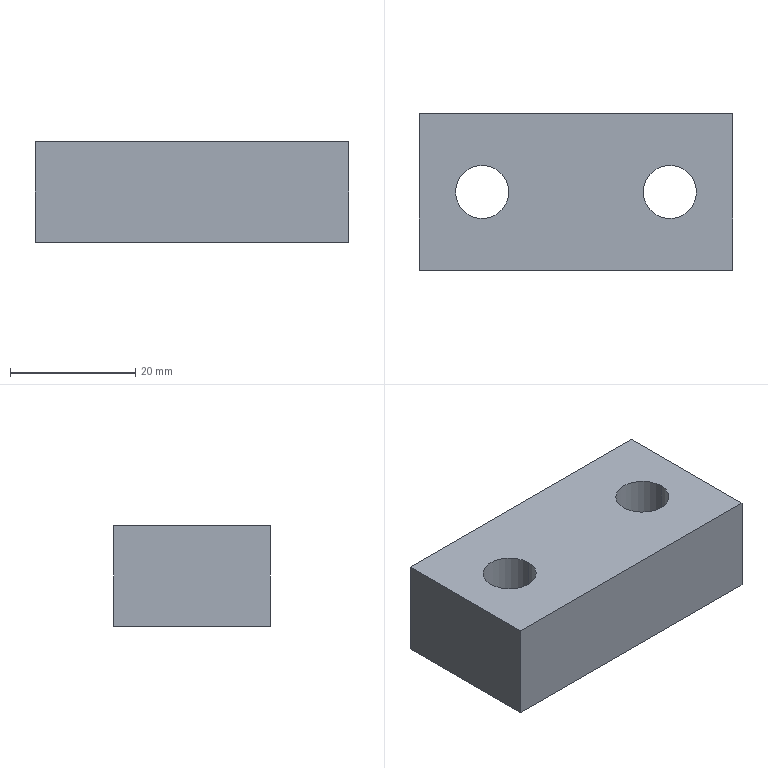Part | SolidWorks | features FlatPattern 1, HoleWzd 1, SMBaseFlange 1, SheetMetal 1 | 1 solid | 10 faces | box 50 x 25 x 16 mm | volume 18184 mm3 | plane 6 | cylinder 4 | commonest cylinder face diameters 8.5 x4
STEP:
#1=CARTESIAN_POINT('',(35.75,-12.5,-16.));
#2=VERTEX_POINT('',#1);
#3=CARTESIAN_POINT('',(44.25,-12.5,-16.));
#4=VERTEX_POINT('',#3);
#5=CARTESIAN_POINT('',(40.,-12.5,-16.));
#6=DIRECTION('',(0.,0.,1.));
#7=DIRECTION('',(1.,0.,0.));
#8=AXIS2_PLACEMENT_3D('',#5,#6,#7);
#9=CIRCLE('',#8,4.25);
#10=EDGE_CURVE('',#2,#4,#9,.T.);
#11=ORIENTED_EDGE('',*,*,#10,.F.);
#12=CARTESIAN_POINT('',(35.75,-12.5,0.));
#13=VERTEX_POINT('',#12);
#14=CARTESIAN_POINT('',(35.75,-12.5,0.));
#15=DIRECTION('',(0.,0.,1.));
#16=VECTOR('',#15,1000.);
#17=LINE('',#14,#16);
#18=EDGE_CURVE('',#2,#13,#17,.T.);
#19=ORIENTED_EDGE('',*,*,#18,.T.);
#20=CARTESIAN_POINT('',(44.25,-12.5,0.));
#21=VERTEX_POINT('',#20);
#22=CARTESIAN_POINT('',(40.,-12.5,0.));
#23=DIRECTION('',(0.,0.,1.));
#24=DIRECTION('',(1.,0.,0.));
#25=AXIS2_PLACEMENT_3D('',#22,#23,#24);
#26=CIRCLE('',#25,4.25);
#27=EDGE_CURVE('',#13,#21,#26,.T.);
#28=ORIENTED_EDGE('',*,*,#27,.T.);
#29=CARTESIAN_POINT('',(44.25,-12.5,0.));
#30=DIRECTION('',(0.,0.,1.));
#31=VECTOR('',#30,1000.);
#32=LINE('',#29,#31);
#33=EDGE_CURVE('',#4,#21,#32,.T.);
#34=ORIENTED_EDGE('',*,*,#33,.F.);
#35=EDGE_LOOP('',(#11,#19,#28,#34));
#36=FACE_OUTER_BOUND('',#35,.T.);
#37=CARTESIAN_POINT('',(40.,-12.5,0.));
#38=DIRECTION('',(0.,0.,1.));
#39=DIRECTION('',(1.,0.,0.));
#40=AXIS2_PLACEMENT_3D('',#37,#38,#39);
#41=CYLINDRICAL_SURFACE('',#40,4.25);
#42=ADVANCED_FACE('',(#36),#41,.F.);
#43=CARTESIAN_POINT('',(5.75,-12.5,-16.));
#44=VERTEX_POINT('',#43);
#45=CARTESIAN_POINT('',(14.25,-12.5,-16.));
#46=VERTEX_POINT('',#45);
#47=CARTESIAN_POINT('',(10.,-12.5,-16.));
#48=DIRECTION('',(0.,0.,1.));
#49=DIRECTION('',(1.,0.,0.));
#50=AXIS2_PLACEMENT_3D('',#47,#48,#49);
#51=CIRCLE('',#50,4.25);
#52=EDGE_CURVE('',#44,#46,#51,.T.);
#53=ORIENTED_EDGE('',*,*,#52,.F.);
#54=CARTESIAN_POINT('',(5.75,-12.5,0.));
#55=VERTEX_POINT('',#54);
#56=CARTESIAN_POINT('',(5.75,-12.5,0.));
#57=DIRECTION('',(0.,0.,1.));
#58=VECTOR('',#57,1000.);
#59=LINE('',#56,#58);
#60=EDGE_CURVE('',#44,#55,#59,.T.);
#61=ORIENTED_EDGE('',*,*,#60,.T.);
#62=CARTESIAN_POINT('',(14.25,-12.5,0.));
#63=VERTEX_POINT('',#62);
#64=CARTESIAN_POINT('',(10.,-12.5,0.));
#65=DIRECTION('',(0.,0.,1.));
#66=DIRECTION('',(1.,0.,0.));
#67=AXIS2_PLACEMENT_3D('',#64,#65,#66);
#68=CIRCLE('',#67,4.25);
#69=EDGE_CURVE('',#55,#63,#68,.T.);
#70=ORIENTED_EDGE('',*,*,#69,.T.);
#71=CARTESIAN_POINT('',(14.25,-12.5,0.));
#72=DIRECTION('',(0.,0.,1.));
#73=VECTOR('',#72,1000.);
#74=LINE('',#71,#73);
#75=EDGE_CURVE('',#46,#63,#74,.T.);
#76=ORIENTED_EDGE('',*,*,#75,.F.);
#77=EDGE_LOOP('',(#53,#61,#70,#76));
#78=FACE_OUTER_BOUND('',#77,.T.);
#79=CARTESIAN_POINT('',(10.,-12.5,0.));
#80=DIRECTION('',(0.,0.,1.));
#81=DIRECTION('',(1.,0.,0.));
#82=AXIS2_PLACEMENT_3D('',#79,#80,#81);
#83=CYLINDRICAL_SURFACE('',#82,4.25);
#84=ADVANCED_FACE('',(#78),#83,.F.);
#85=CARTESIAN_POINT('',(0.,0.,0.));
#86=VERTEX_POINT('',#85);
#87=CARTESIAN_POINT('',(0.,-25.,0.));
#88=VERTEX_POINT('',#87);
#89=CARTESIAN_POINT('',(0.,0.,0.));
#90=DIRECTION('',(0.,-1.,0.));
#91=VECTOR('',#90,1000.);
#92=LINE('',#89,#91);
#93=EDGE_CURVE('',#86,#88,#92,.T.);
#94=ORIENTED_EDGE('',*,*,#93,.F.);
#95=CARTESIAN_POINT('',(0.,0.,-16.));
#96=VERTEX_POINT('',#95);
#97=CARTESIAN_POINT('',(0.,0.,-16.));
#98=DIRECTION('',(0.,0.,1.));
#99=VECTOR('',#98,1000.);
#100=LINE('',#97,#99);
#101=EDGE_CURVE('',#96,#86,#100,.T.);
#102=ORIENTED_EDGE('',*,*,#101,.F.);
#103=CARTESIAN_POINT('',(0.,-25.,-16.));
#104=VERTEX_POINT('',#103);
#105=CARTESIAN_POINT('',(0.,0.,-16.));
#106=DIRECTION('',(0.,-1.,0.));
#107=VECTOR('',#106,1000.);
#108=LINE('',#105,#107);
#109=EDGE_CURVE('',#96,#104,#108,.T.);
#110=ORIENTED_EDGE('',*,*,#109,.T.);
#111=CARTESIAN_POINT('',(0.,-25.,-16.));
#112=DIRECTION('',(0.,0.,1.));
#113=VECTOR('',#112,1000.);
#114=LINE('',#111,#113);
#115=EDGE_CURVE('',#104,#88,#114,.T.);
#116=ORIENTED_EDGE('',*,*,#115,.T.);
#117=EDGE_LOOP('',(#94,#102,#110,#116));
#118=FACE_OUTER_BOUND('',#117,.T.);
#119=CARTESIAN_POINT('',(0.,0.,-16.));
#120=DIRECTION('',(-1.,0.,0.));
#121=DIRECTION('',(0.,-1.,0.));
#122=AXIS2_PLACEMENT_3D('',#119,#120,#121);
#123=PLANE('',#122);
#124=ADVANCED_FACE('',(#118),#123,.T.);
#125=CARTESIAN_POINT('',(50.,0.,0.));
#126=VERTEX_POINT('',#125);
#127=CARTESIAN_POINT('',(0.,0.,0.));
#128=DIRECTION('',(-1.,0.,0.));
#129=VECTOR('',#128,1000.);
#130=LINE('',#127,#129);
#131=EDGE_CURVE('',#126,#86,#130,.T.);
#132=ORIENTED_EDGE('',*,*,#131,.F.);
#133=CARTESIAN_POINT('',(50.,0.,-16.));
#134=VERTEX_POINT('',#133);
#135=CARTESIAN_POINT('',(50.,0.,-16.));
#136=DIRECTION('',(0.,0.,1.));
#137=VECTOR('',#136,1000.);
#138=LINE('',#135,#137);
#139=EDGE_CURVE('',#134,#126,#138,.T.);
#140=ORIENTED_EDGE('',*,*,#139,.F.);
#141=CARTESIAN_POINT('',(0.,0.,-16.));
#142=DIRECTION('',(-1.,0.,0.));
#143=VECTOR('',#142,1000.);
#144=LINE('',#141,#143);
#145=EDGE_CURVE('',#134,#96,#144,.T.);
#146=ORIENTED_EDGE('',*,*,#145,.T.);
#147=ORIENTED_EDGE('',*,*,#101,.T.);
#148=EDGE_LOOP('',(#132,#140,#146,#147));
#149=FACE_OUTER_BOUND('',#148,.T.);
#150=CARTESIAN_POINT('',(0.,0.,-16.));
#151=DIRECTION('',(0.,1.,0.));
#152=DIRECTION('',(0.,0.,1.));
#153=AXIS2_PLACEMENT_3D('',#150,#151,#152);
#154=PLANE('',#153);
#155=ADVANCED_FACE('',(#149),#154,.T.);
#156=CARTESIAN_POINT('',(50.,-25.,0.));
#157=VERTEX_POINT('',#156);
#158=CARTESIAN_POINT('',(50.,0.,0.));
#159=DIRECTION('',(0.,1.,0.));
#160=VECTOR('',#159,1000.);
#161=LINE('',#158,#160);
#162=EDGE_CURVE('',#157,#126,#161,.T.);
#163=ORIENTED_EDGE('',*,*,#162,.F.);
#164=CARTESIAN_POINT('',(50.,-25.,-16.));
#165=VERTEX_POINT('',#164);
#166=CARTESIAN_POINT('',(50.,-25.,-16.));
#167=DIRECTION('',(0.,0.,1.));
#168=VECTOR('',#167,1000.);
#169=LINE('',#166,#168);
#170=EDGE_CURVE('',#165,#157,#169,.T.);
#171=ORIENTED_EDGE('',*,*,#170,.F.);
#172=CARTESIAN_POINT('',(50.,0.,-16.));
#173=DIRECTION('',(0.,1.,0.));
#174=VECTOR('',#173,1000.);
#175=LINE('',#172,#174);
#176=EDGE_CURVE('',#165,#134,#175,.T.);
#177=ORIENTED_EDGE('',*,*,#176,.T.);
#178=ORIENTED_EDGE('',*,*,#139,.T.);
#179=EDGE_LOOP('',(#163,#171,#177,#178));
#180=FACE_OUTER_BOUND('',#179,.T.);
#181=CARTESIAN_POINT('',(50.,0.,-16.));
#182=DIRECTION('',(1.,0.,0.));
#183=DIRECTION('',(0.,0.,-1.));
#184=AXIS2_PLACEMENT_3D('',#181,#182,#183);
#185=PLANE('',#184);
#186=ADVANCED_FACE('',(#180),#185,.T.);
#187=CARTESIAN_POINT('',(0.,-25.,0.));
#188=DIRECTION('',(1.,0.,0.));
#189=VECTOR('',#188,1000.);
#190=LINE('',#187,#189);
#191=EDGE_CURVE('',#88,#157,#190,.T.);
#192=ORIENTED_EDGE('',*,*,#191,.F.);
#193=ORIENTED_EDGE('',*,*,#115,.F.);
#194=CARTESIAN_POINT('',(0.,-25.,-16.));
#195=DIRECTION('',(1.,0.,0.));
#196=VECTOR('',#195,1000.);
#197=LINE('',#194,#196);
#198=EDGE_CURVE('',#104,#165,#197,.T.);
#199=ORIENTED_EDGE('',*,*,#198,.T.);
#200=ORIENTED_EDGE('',*,*,#170,.T.);
#201=EDGE_LOOP('',(#192,#193,#199,#200));
#202=FACE_OUTER_BOUND('',#201,.T.);
#203=CARTESIAN_POINT('',(0.,-25.,-16.));
#204=DIRECTION('',(0.,-1.,0.));
#205=DIRECTION('',(0.,0.,-1.));
#206=AXIS2_PLACEMENT_3D('',#203,#204,#205);
#207=PLANE('',#206);
#208=ADVANCED_FACE('',(#202),#207,.T.);
#209=CARTESIAN_POINT('',(40.,-12.5,-16.));
#210=DIRECTION('',(0.,0.,1.));
#211=DIRECTION('',(1.,0.,0.));
#212=AXIS2_PLACEMENT_3D('',#209,#210,#211);
#213=CIRCLE('',#212,4.25);
#214=EDGE_CURVE('',#4,#2,#213,.T.);
#215=ORIENTED_EDGE('',*,*,#214,.T.);
#216=ORIENTED_EDGE('',*,*,#10,.T.);
#217=EDGE_LOOP('',(#215,#216));
#218=FACE_BOUND('',#217,.T.);
#219=CARTESIAN_POINT('',(10.,-12.5,-16.));
#220=DIRECTION('',(0.,0.,1.));
#221=DIRECTION('',(1.,0.,0.));
#222=AXIS2_PLACEMENT_3D('',#219,#220,#221);
#223=CIRCLE('',#222,4.25);
#224=EDGE_CURVE('',#46,#44,#223,.T.);
#225=ORIENTED_EDGE('',*,*,#224,.T.);
#226=ORIENTED_EDGE('',*,*,#52,.T.);
#227=EDGE_LOOP('',(#225,#226));
#228=FACE_BOUND('',#227,.T.);
#229=ORIENTED_EDGE('',*,*,#109,.F.);
#230=ORIENTED_EDGE('',*,*,#145,.F.);
#231=ORIENTED_EDGE('',*,*,#176,.F.);
#232=ORIENTED_EDGE('',*,*,#198,.F.);
#233=EDGE_LOOP('',(#229,#230,#231,#232));
#234=FACE_OUTER_BOUND('',#233,.T.);
#235=CARTESIAN_POINT('',(0.,0.,-16.));
#236=DIRECTION('',(0.,0.,1.));
#237=DIRECTION('',(1.,0.,0.));
#238=AXIS2_PLACEMENT_3D('',#235,#236,#237);
#239=PLANE('',#238);
#240=ADVANCED_FACE('',(#218,#228,#234),#239,.F.);
#241=CARTESIAN_POINT('',(40.,-12.5,0.));
#242=DIRECTION('',(0.,0.,1.));
#243=DIRECTION('',(1.,0.,0.));
#244=AXIS2_PLACEMENT_3D('',#241,#242,#243);
#245=CIRCLE('',#244,4.25);
#246=EDGE_CURVE('',#21,#13,#245,.T.);
#247=ORIENTED_EDGE('',*,*,#246,.F.);
#248=ORIENTED_EDGE('',*,*,#27,.F.);
#249=EDGE_LOOP('',(#247,#248));
#250=FACE_BOUND('',#249,.T.);
#251=CARTESIAN_POINT('',(10.,-12.5,0.));
#252=DIRECTION('',(0.,0.,1.));
#253=DIRECTION('',(1.,0.,0.));
#254=AXIS2_PLACEMENT_3D('',#251,#252,#253);
#255=CIRCLE('',#254,4.25);
#256=EDGE_CURVE('',#63,#55,#255,.T.);
#257=ORIENTED_EDGE('',*,*,#256,.F.);
#258=ORIENTED_EDGE('',*,*,#69,.F.);
#259=EDGE_LOOP('',(#257,#258));
#260=FACE_BOUND('',#259,.T.);
#261=ORIENTED_EDGE('',*,*,#93,.T.);
#262=ORIENTED_EDGE('',*,*,#191,.T.);
#263=ORIENTED_EDGE('',*,*,#162,.T.);
#264=ORIENTED_EDGE('',*,*,#131,.T.);
#265=EDGE_LOOP('',(#261,#262,#263,#264));
#266=FACE_OUTER_BOUND('',#265,.T.);
#267=CARTESIAN_POINT('',(0.,0.,0.));
#268=DIRECTION('',(0.,0.,1.));
#269=DIRECTION('',(1.,0.,0.));
#270=AXIS2_PLACEMENT_3D('',#267,#268,#269);
#271=PLANE('',#270);
#272=ADVANCED_FACE('',(#250,#260,#266),#271,.T.);
#273=ORIENTED_EDGE('',*,*,#60,.F.);
#274=ORIENTED_EDGE('',*,*,#224,.F.);
#275=ORIENTED_EDGE('',*,*,#75,.T.);
#276=ORIENTED_EDGE('',*,*,#256,.T.);
#277=EDGE_LOOP('',(#273,#274,#275,#276));
#278=FACE_OUTER_BOUND('',#277,.T.);
#279=CARTESIAN_POINT('',(10.,-12.5,0.));
#280=DIRECTION('',(0.,0.,1.));
#281=DIRECTION('',(1.,0.,0.));
#282=AXIS2_PLACEMENT_3D('',#279,#280,#281);
#283=CYLINDRICAL_SURFACE('',#282,4.25);
#284=ADVANCED_FACE('',(#278),#283,.F.);
#285=ORIENTED_EDGE('',*,*,#18,.F.);
#286=ORIENTED_EDGE('',*,*,#214,.F.);
#287=ORIENTED_EDGE('',*,*,#33,.T.);
#288=ORIENTED_EDGE('',*,*,#246,.T.);
#289=EDGE_LOOP('',(#285,#286,#287,#288));
#290=FACE_OUTER_BOUND('',#289,.T.);
#291=CARTESIAN_POINT('',(40.,-12.5,0.));
#292=DIRECTION('',(0.,0.,1.));
#293=DIRECTION('',(1.,0.,0.));
#294=AXIS2_PLACEMENT_3D('',#291,#292,#293);
#295=CYLINDRICAL_SURFACE('',#294,4.25);
#296=ADVANCED_FACE('',(#290),#295,.F.);
#297=CLOSED_SHELL('',(#42,#84,#124,#155,#186,#208,#240,#272,#284,#296));
#298=MANIFOLD_SOLID_BREP('',#297);
#299=CARTESIAN_POINT('',(0.,0.,0.));
#300=DIRECTION('',(0.,0.,1.));
#301=DIRECTION('',(1.,0.,0.));
#302=AXIS2_PLACEMENT_3D('',#299,#300,#301);
#303=(LENGTH_UNIT()NAMED_UNIT(*)SI_UNIT(.MILLI.,.METRE.));
#304=UNCERTAINTY_MEASURE_WITH_UNIT(LENGTH_MEASURE(0.00001),#303,'','');
#305=(NAMED_UNIT(*)PLANE_ANGLE_UNIT()SI_UNIT($,.RADIAN.));
#306=(NAMED_UNIT(*)SI_UNIT($,.STERADIAN.)SOLID_ANGLE_UNIT());
#307=(GEOMETRIC_REPRESENTATION_CONTEXT(3)GLOBAL_UNCERTAINTY_ASSIGNED_CONTEXT((#304))GLOBAL_UNIT_ASSIGNED_CONTEXT((#303,#305,#306))REPRESENTATION_CONTEXT('',''));
#308=ADVANCED_BREP_SHAPE_REPRESENTATION('',(#298,#302),#307);